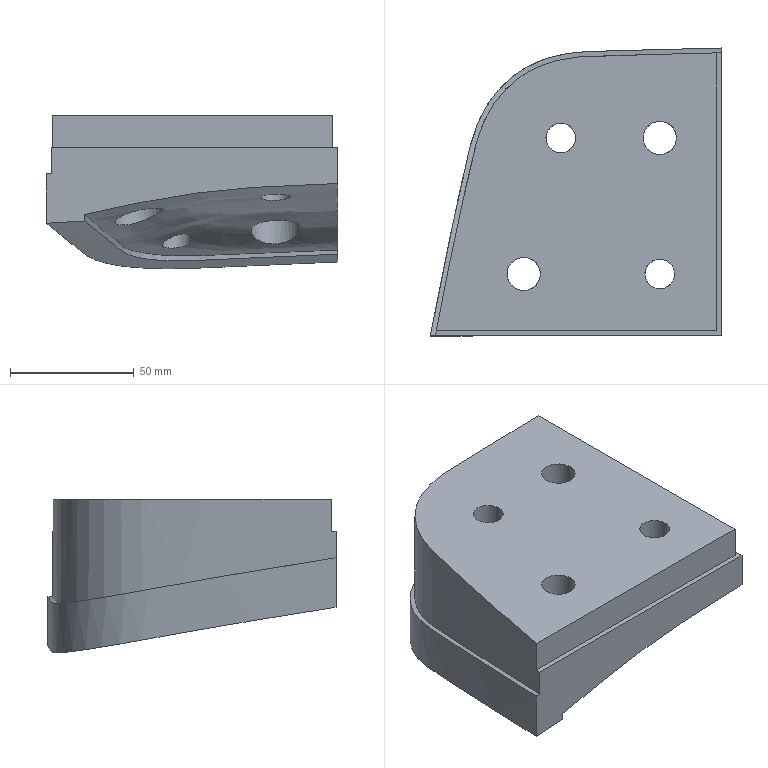Part | NX | features solid 2 | 1 solid | 20 faces | box 117.74 x 116.436 x 62.135 mm | volume 476643 mm3 | plane 8 | spline 6 | cylinder 6 | commonest cylinder face diameters 12 x2 13.5 x2 20 x2